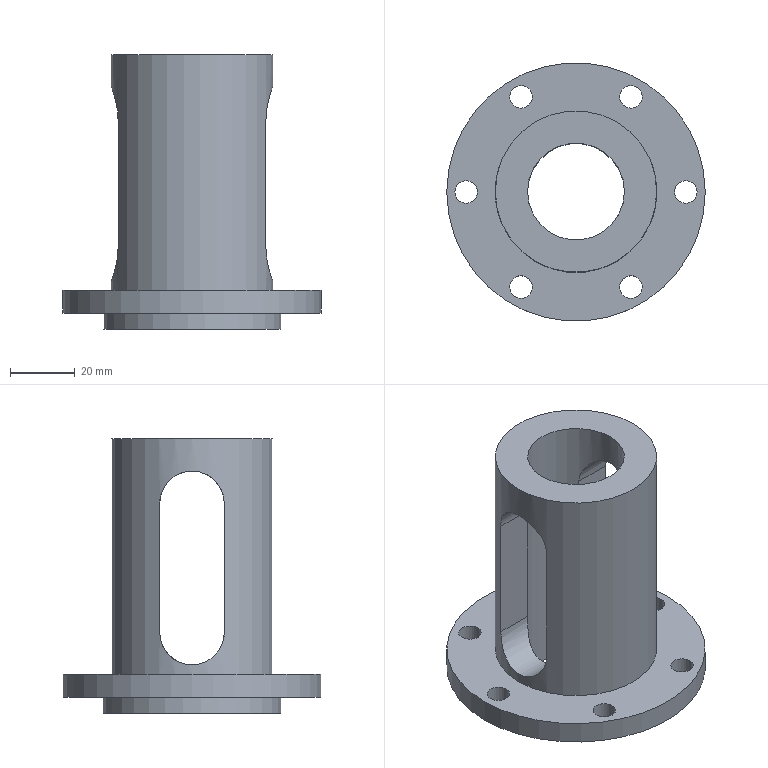CAM job | NX | 3+2 milling, drilling | part box 80 x 80 x 85 mm
Tools:
number,name,description,diameter,corner_radius,flute_length,length,flutes
4,D16R0.8,Milling Tool-5 Parameters,16.0,0.8,50.0,75.0,2
1,ZXZ,Milling Tool-5 Parameters,6.0,0.0,50.0,75.0,2
2,7.0ZT,Drilling Tool,7.0,0.0,35.0,50.0,2
5,D6A45,Milling Tool-5 Parameters,6.0,0.0,3.0,3.0,2
Operations:
program,operation,operation_type,tool,method,geometry_group,spindle_rpm,surface_speed,feed_per_tooth,feed_cut,feed_plunge,cut_length_mm,path_length_mm,cut_time_min,machine_time_min
1,ZLEVEL_PROFILE,ZLevelMilling,D16R0.8,METHOD,A,2200.0,110.0,0.5,2200.0,1000.0,4675.179,4771.568,2.143,2.153
1,PROFILE_3D,PlanarMilling,D6A45,METHOD,A,7500.0,141.0,0.0833,1250.0,100.0,153.442,245.036,0.1228,0.1319
2,DRILLING,Operation,ZXZ,METHOD,B,3000.0,56.0,0.0333,200.0,0.0,24.0,303.661,0.12,0.148
2,DRILLING_COPY,Operation,7.0ZT,METHOD,B,2000.0,43.0,0.05,200.0,0.0,81.618,418.897,0.4081,0.4418